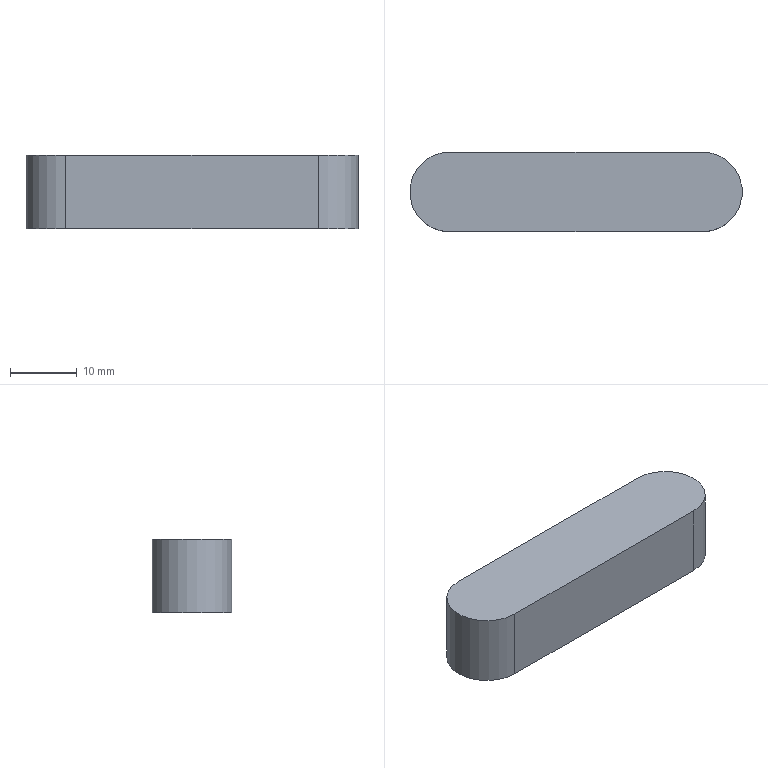Part | NX | features DATUM_CSYS 2, EXTRUDE 1, SKETCH 1 | 1 solid | 6 faces | box 50 x 12 x 11 mm | volume 6260 mm3 | plane 4 | cylinder 2 | commonest cylinder face diameters 12 x2
STEP:
#1=CARTESIAN_POINT('',(-38.,6.,0.));
#2=VERTEX_POINT('',#1);
#3=CARTESIAN_POINT('',(-38.,-6.,0.));
#4=VERTEX_POINT('',#3);
#5=CARTESIAN_POINT('',(-38.,0.,0.));
#6=DIRECTION('',(0.,0.,1.));
#7=DIRECTION('',(1.,0.,0.));
#8=AXIS2_PLACEMENT_3D('',#5,#6,#7);
#9=CIRCLE('',#8,6.);
#10=EDGE_CURVE('',#2,#4,#9,.T.);
#11=ORIENTED_EDGE('',*,*,#10,.T.);
#12=CARTESIAN_POINT('',(-38.,-6.,11.));
#13=VERTEX_POINT('',#12);
#14=CARTESIAN_POINT('',(-38.,-6.,11.));
#15=DIRECTION('',(0.,0.,-1.));
#16=VECTOR('',#15,1000.);
#17=LINE('',#14,#16);
#18=EDGE_CURVE('',#13,#4,#17,.T.);
#19=ORIENTED_EDGE('',*,*,#18,.F.);
#20=CARTESIAN_POINT('',(-38.,6.,11.));
#21=VERTEX_POINT('',#20);
#22=CARTESIAN_POINT('',(-38.,0.,11.));
#23=DIRECTION('',(0.,0.,1.));
#24=DIRECTION('',(1.,0.,0.));
#25=AXIS2_PLACEMENT_3D('',#22,#23,#24);
#26=CIRCLE('',#25,6.);
#27=EDGE_CURVE('',#21,#13,#26,.T.);
#28=ORIENTED_EDGE('',*,*,#27,.F.);
#29=CARTESIAN_POINT('',(-38.,6.,11.));
#30=DIRECTION('',(0.,0.,-1.));
#31=VECTOR('',#30,1000.);
#32=LINE('',#29,#31);
#33=EDGE_CURVE('',#21,#2,#32,.T.);
#34=ORIENTED_EDGE('',*,*,#33,.T.);
#35=EDGE_LOOP('',(#11,#19,#28,#34));
#36=FACE_BOUND('',#35,.T.);
#37=CARTESIAN_POINT('',(-38.,0.,11.));
#38=DIRECTION('',(0.,0.,-1.));
#39=DIRECTION('',(-1.,0.,0.));
#40=AXIS2_PLACEMENT_3D('',#37,#38,#39);
#41=CYLINDRICAL_SURFACE('',#40,6.);
#42=ADVANCED_FACE('',(#36),#41,.T.);
#43=CARTESIAN_POINT('',(0.,-6.,0.));
#44=VERTEX_POINT('',#43);
#45=CARTESIAN_POINT('',(-38.,-6.,0.));
#46=DIRECTION('',(1.,0.,0.));
#47=VECTOR('',#46,1000.);
#48=LINE('',#45,#47);
#49=EDGE_CURVE('',#4,#44,#48,.T.);
#50=ORIENTED_EDGE('',*,*,#49,.T.);
#51=CARTESIAN_POINT('',(0.,-6.,11.));
#52=VERTEX_POINT('',#51);
#53=CARTESIAN_POINT('',(0.,-6.,11.));
#54=DIRECTION('',(0.,0.,-1.));
#55=VECTOR('',#54,1000.);
#56=LINE('',#53,#55);
#57=EDGE_CURVE('',#52,#44,#56,.T.);
#58=ORIENTED_EDGE('',*,*,#57,.F.);
#59=CARTESIAN_POINT('',(-38.,-6.,11.));
#60=DIRECTION('',(1.,0.,0.));
#61=VECTOR('',#60,1000.);
#62=LINE('',#59,#61);
#63=EDGE_CURVE('',#13,#52,#62,.T.);
#64=ORIENTED_EDGE('',*,*,#63,.F.);
#65=ORIENTED_EDGE('',*,*,#18,.T.);
#66=EDGE_LOOP('',(#50,#58,#64,#65));
#67=FACE_BOUND('',#66,.T.);
#68=CARTESIAN_POINT('',(-38.,-6.,11.));
#69=DIRECTION('',(0.,1.,0.));
#70=DIRECTION('',(-1.,0.,0.));
#71=AXIS2_PLACEMENT_3D('',#68,#69,#70);
#72=PLANE('',#71);
#73=ADVANCED_FACE('',(#67),#72,.F.);
#74=CARTESIAN_POINT('',(0.,6.,0.));
#75=VERTEX_POINT('',#74);
#76=CARTESIAN_POINT('',(0.,0.,0.));
#77=DIRECTION('',(0.,0.,1.));
#78=DIRECTION('',(1.,0.,0.));
#79=AXIS2_PLACEMENT_3D('',#76,#77,#78);
#80=CIRCLE('',#79,6.);
#81=EDGE_CURVE('',#44,#75,#80,.T.);
#82=ORIENTED_EDGE('',*,*,#81,.T.);
#83=CARTESIAN_POINT('',(0.,6.,11.));
#84=VERTEX_POINT('',#83);
#85=CARTESIAN_POINT('',(0.,6.,11.));
#86=DIRECTION('',(0.,0.,-1.));
#87=VECTOR('',#86,1000.);
#88=LINE('',#85,#87);
#89=EDGE_CURVE('',#84,#75,#88,.T.);
#90=ORIENTED_EDGE('',*,*,#89,.F.);
#91=CARTESIAN_POINT('',(0.,0.,11.));
#92=DIRECTION('',(0.,0.,1.));
#93=DIRECTION('',(1.,0.,0.));
#94=AXIS2_PLACEMENT_3D('',#91,#92,#93);
#95=CIRCLE('',#94,6.);
#96=EDGE_CURVE('',#52,#84,#95,.T.);
#97=ORIENTED_EDGE('',*,*,#96,.F.);
#98=ORIENTED_EDGE('',*,*,#57,.T.);
#99=EDGE_LOOP('',(#82,#90,#97,#98));
#100=FACE_BOUND('',#99,.T.);
#101=CARTESIAN_POINT('',(0.,0.,11.));
#102=DIRECTION('',(0.,0.,-1.));
#103=DIRECTION('',(-1.,0.,0.));
#104=AXIS2_PLACEMENT_3D('',#101,#102,#103);
#105=CYLINDRICAL_SURFACE('',#104,6.);
#106=ADVANCED_FACE('',(#100),#105,.T.);
#107=CARTESIAN_POINT('',(0.,6.,0.));
#108=DIRECTION('',(-1.,0.,0.));
#109=VECTOR('',#108,1000.);
#110=LINE('',#107,#109);
#111=EDGE_CURVE('',#75,#2,#110,.T.);
#112=ORIENTED_EDGE('',*,*,#111,.T.);
#113=ORIENTED_EDGE('',*,*,#33,.F.);
#114=CARTESIAN_POINT('',(0.,6.,11.));
#115=DIRECTION('',(-1.,0.,0.));
#116=VECTOR('',#115,1000.);
#117=LINE('',#114,#116);
#118=EDGE_CURVE('',#84,#21,#117,.T.);
#119=ORIENTED_EDGE('',*,*,#118,.F.);
#120=ORIENTED_EDGE('',*,*,#89,.T.);
#121=EDGE_LOOP('',(#112,#113,#119,#120));
#122=FACE_BOUND('',#121,.T.);
#123=CARTESIAN_POINT('',(0.,6.,11.));
#124=DIRECTION('',(0.,-1.,0.));
#125=DIRECTION('',(1.,0.,0.));
#126=AXIS2_PLACEMENT_3D('',#123,#124,#125);
#127=PLANE('',#126);
#128=ADVANCED_FACE('',(#122),#127,.F.);
#129=ORIENTED_EDGE('',*,*,#27,.T.);
#130=ORIENTED_EDGE('',*,*,#63,.T.);
#131=ORIENTED_EDGE('',*,*,#96,.T.);
#132=ORIENTED_EDGE('',*,*,#118,.T.);
#133=EDGE_LOOP('',(#129,#130,#131,#132));
#134=FACE_BOUND('',#133,.T.);
#135=CARTESIAN_POINT('',(-38.,0.,11.));
#136=DIRECTION('',(0.,0.,1.));
#137=DIRECTION('',(1.,0.,0.));
#138=AXIS2_PLACEMENT_3D('',#135,#136,#137);
#139=PLANE('',#138);
#140=ADVANCED_FACE('',(#134),#139,.T.);
#141=ORIENTED_EDGE('',*,*,#10,.F.);
#142=ORIENTED_EDGE('',*,*,#111,.F.);
#143=ORIENTED_EDGE('',*,*,#81,.F.);
#144=ORIENTED_EDGE('',*,*,#49,.F.);
#145=EDGE_LOOP('',(#141,#142,#143,#144));
#146=FACE_BOUND('',#145,.T.);
#147=CARTESIAN_POINT('',(-38.,0.,0.));
#148=DIRECTION('',(0.,0.,1.));
#149=DIRECTION('',(1.,0.,0.));
#150=AXIS2_PLACEMENT_3D('',#147,#148,#149);
#151=PLANE('',#150);
#152=ADVANCED_FACE('',(#146),#151,.F.);
#153=CLOSED_SHELL('',(#42,#73,#106,#128,#140,#152));
#154=MANIFOLD_SOLID_BREP('',#153);
#155=(LENGTH_UNIT()NAMED_UNIT(*)SI_UNIT(.MILLI.,.METRE.));
#156=UNCERTAINTY_MEASURE_WITH_UNIT(LENGTH_MEASURE(0.00001),#155,'','');
#157=(NAMED_UNIT(*)PLANE_ANGLE_UNIT()SI_UNIT($,.RADIAN.));
#158=(NAMED_UNIT(*)SI_UNIT($,.STERADIAN.)SOLID_ANGLE_UNIT());
#159=(GEOMETRIC_REPRESENTATION_CONTEXT(3)GLOBAL_UNCERTAINTY_ASSIGNED_CONTEXT((#156))GLOBAL_UNIT_ASSIGNED_CONTEXT((#155,#157,#158))REPRESENTATION_CONTEXT('',''));
#160=ADVANCED_BREP_SHAPE_REPRESENTATION('',(#154),#159);